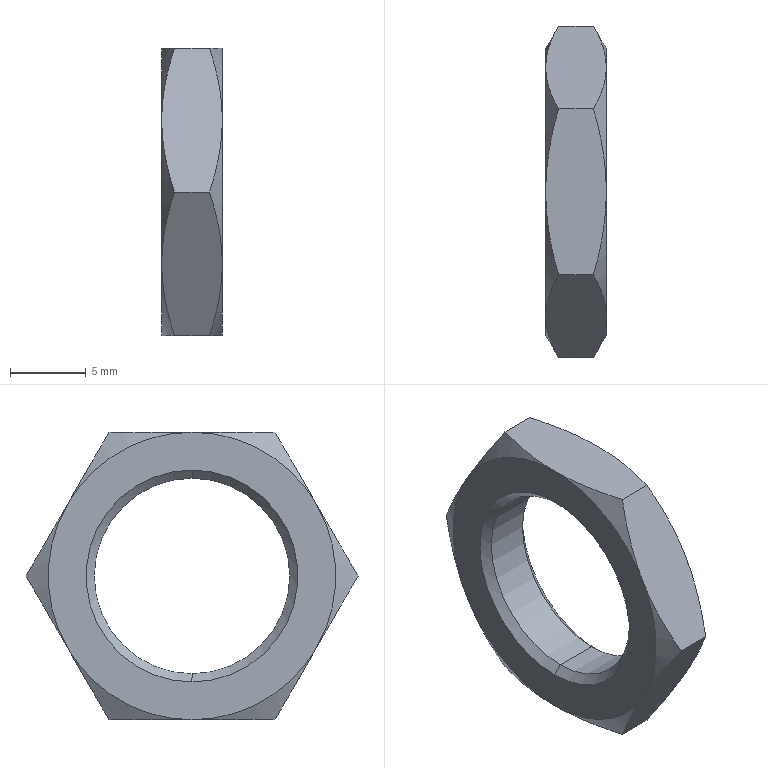Part | SolidWorks | features RefAxis 3, RevCut 2, 3DProfileFeature 1, Extrusion 1 | 1 solid | 26 faces | box 4 x 21.939 x 19 mm | volume 699.231 mm3 | cone 16 | plane 8 | cylinder 2 | commonest cylinder face diameters 12.917 x2
STEP:
#1=CARTESIAN_POINT('',(3.459,0.,6.458));
#2=VERTEX_POINT('',#1);
#3=CARTESIAN_POINT('',(3.459,0.,-6.458));
#4=VERTEX_POINT('',#3);
#5=CARTESIAN_POINT('',(3.459,0.,0.));
#6=DIRECTION('',(1.,0.,0.));
#7=DIRECTION('',(0.,0.,-1.));
#8=AXIS2_PLACEMENT_3D('',#5,#6,#7);
#9=CIRCLE('',#8,6.458);
#10=EDGE_CURVE('',#2,#4,#9,.T.);
#11=ORIENTED_EDGE('',*,*,#10,.F.);
#12=CARTESIAN_POINT('',(4.,0.,7.));
#13=VERTEX_POINT('',#12);
#14=CARTESIAN_POINT('',(4.,0.,7.));
#15=DIRECTION('',(0.7071,0.,0.7071));
#16=VECTOR('',#15,1000.);
#17=LINE('',#14,#16);
#18=EDGE_CURVE('',#2,#13,#17,.T.);
#19=ORIENTED_EDGE('',*,*,#18,.T.);
#20=CARTESIAN_POINT('',(4.,0.,-7.));
#21=VERTEX_POINT('',#20);
#22=CARTESIAN_POINT('',(4.,0.,0.));
#23=DIRECTION('',(1.,0.,0.));
#24=DIRECTION('',(0.,0.,-1.));
#25=AXIS2_PLACEMENT_3D('',#22,#23,#24);
#26=CIRCLE('',#25,7.);
#27=EDGE_CURVE('',#13,#21,#26,.T.);
#28=ORIENTED_EDGE('',*,*,#27,.T.);
#29=CARTESIAN_POINT('',(4.,0.,-7.));
#30=DIRECTION('',(0.7071,0.,-0.7071));
#31=VECTOR('',#30,1000.);
#32=LINE('',#29,#31);
#33=EDGE_CURVE('',#4,#21,#32,.T.);
#34=ORIENTED_EDGE('',*,*,#33,.F.);
#35=EDGE_LOOP('',(#11,#19,#28,#34));
#36=FACE_OUTER_BOUND('',#35,.T.);
#37=CARTESIAN_POINT('',(4.,0.,0.));
#38=DIRECTION('',(1.,0.,0.));
#39=DIRECTION('',(0.,0.,-1.));
#40=AXIS2_PLACEMENT_3D('',#37,#38,#39);
#41=CONICAL_SURFACE('',#40,7.,0.7854);
#42=ADVANCED_FACE('',(#36),#41,.F.);
#43=CARTESIAN_POINT('',(0.5415,0.,6.458));
#44=VERTEX_POINT('',#43);
#45=CARTESIAN_POINT('',(0.5415,0.,-6.458));
#46=VERTEX_POINT('',#45);
#47=CARTESIAN_POINT('',(0.5415,0.,0.));
#48=DIRECTION('',(1.,0.,0.));
#49=DIRECTION('',(0.,0.,-1.));
#50=AXIS2_PLACEMENT_3D('',#47,#48,#49);
#51=CIRCLE('',#50,6.458);
#52=EDGE_CURVE('',#44,#46,#51,.T.);
#53=ORIENTED_EDGE('',*,*,#52,.F.);
#54=CARTESIAN_POINT('',(4.,0.,6.458));
#55=DIRECTION('',(1.,0.,0.));
#56=VECTOR('',#55,1000.);
#57=LINE('',#54,#56);
#58=EDGE_CURVE('',#44,#2,#57,.T.);
#59=ORIENTED_EDGE('',*,*,#58,.T.);
#60=ORIENTED_EDGE('',*,*,#10,.T.);
#61=CARTESIAN_POINT('',(4.,0.,-6.458));
#62=DIRECTION('',(1.,0.,0.));
#63=VECTOR('',#62,1000.);
#64=LINE('',#61,#63);
#65=EDGE_CURVE('',#46,#4,#64,.T.);
#66=ORIENTED_EDGE('',*,*,#65,.F.);
#67=EDGE_LOOP('',(#53,#59,#60,#66));
#68=FACE_OUTER_BOUND('',#67,.T.);
#69=CARTESIAN_POINT('',(4.,0.,0.));
#70=DIRECTION('',(1.,0.,0.));
#71=DIRECTION('',(0.,0.,-1.));
#72=AXIS2_PLACEMENT_3D('',#69,#70,#71);
#73=CYLINDRICAL_SURFACE('',#72,6.458);
#74=ADVANCED_FACE('',(#68),#73,.F.);
#75=ORIENTED_EDGE('',*,*,#52,.T.);
#76=CARTESIAN_POINT('',(0.,0.,-7.));
#77=VERTEX_POINT('',#76);
#78=CARTESIAN_POINT('',(0.5415,0.,-6.458));
#79=DIRECTION('',(-0.7071,0.,-0.7071));
#80=VECTOR('',#79,1000.);
#81=LINE('',#78,#80);
#82=EDGE_CURVE('',#46,#77,#81,.T.);
#83=ORIENTED_EDGE('',*,*,#82,.T.);
#84=CARTESIAN_POINT('',(0.,0.,7.));
#85=VERTEX_POINT('',#84);
#86=CARTESIAN_POINT('',(0.,0.,0.));
#87=DIRECTION('',(1.,0.,0.));
#88=DIRECTION('',(0.,0.,-1.));
#89=AXIS2_PLACEMENT_3D('',#86,#87,#88);
#90=CIRCLE('',#89,7.);
#91=EDGE_CURVE('',#85,#77,#90,.T.);
#92=ORIENTED_EDGE('',*,*,#91,.F.);
#93=CARTESIAN_POINT('',(0.5415,0.,6.458));
#94=DIRECTION('',(-0.7071,0.,0.7071));
#95=VECTOR('',#94,1000.);
#96=LINE('',#93,#95);
#97=EDGE_CURVE('',#44,#85,#96,.T.);
#98=ORIENTED_EDGE('',*,*,#97,.F.);
#99=EDGE_LOOP('',(#75,#83,#92,#98));
#100=FACE_OUTER_BOUND('',#99,.T.);
#101=CARTESIAN_POINT('',(0.5415,0.,0.));
#102=DIRECTION('',(-1.,0.,0.));
#103=DIRECTION('',(0.,0.,1.));
#104=AXIS2_PLACEMENT_3D('',#101,#102,#103);
#105=CONICAL_SURFACE('',#104,6.458,0.7854);
#106=ADVANCED_FACE('',(#100),#105,.F.);
#107=CARTESIAN_POINT('',(4.,0.,0.));
#108=DIRECTION('',(1.,0.,0.));
#109=DIRECTION('',(0.,0.,-1.));
#110=AXIS2_PLACEMENT_3D('',#107,#108,#109);
#111=CIRCLE('',#110,7.);
#112=EDGE_CURVE('',#21,#13,#111,.T.);
#113=ORIENTED_EDGE('',*,*,#112,.F.);
#114=ORIENTED_EDGE('',*,*,#27,.F.);
#115=EDGE_LOOP('',(#113,#114));
#116=FACE_BOUND('',#115,.T.);
#117=CARTESIAN_POINT('',(4.,0.,-9.5));
#118=VERTEX_POINT('',#117);
#119=CARTESIAN_POINT('',(4.,-8.227,-4.75));
#120=VERTEX_POINT('',#119);
#121=CARTESIAN_POINT('',(4.,0.,0.));
#122=DIRECTION('',(-1.,0.,0.));
#123=DIRECTION('',(0.,0.,-1.));
#124=AXIS2_PLACEMENT_3D('',#121,#122,#123);
#125=CIRCLE('',#124,9.5);
#126=EDGE_CURVE('',#118,#120,#125,.T.);
#127=ORIENTED_EDGE('',*,*,#126,.F.);
#128=CARTESIAN_POINT('',(4.,8.227,-4.75));
#129=VERTEX_POINT('',#128);
#130=CARTESIAN_POINT('',(4.,0.,0.));
#131=DIRECTION('',(1.,0.,0.));
#132=DIRECTION('',(0.,0.,-1.));
#133=AXIS2_PLACEMENT_3D('',#130,#131,#132);
#134=CIRCLE('',#133,9.5);
#135=EDGE_CURVE('',#118,#129,#134,.T.);
#136=ORIENTED_EDGE('',*,*,#135,.T.);
#137=CARTESIAN_POINT('',(4.,8.227,4.75));
#138=VERTEX_POINT('',#137);
#139=CARTESIAN_POINT('',(4.,0.,0.));
#140=DIRECTION('',(-1.,0.,0.));
#141=DIRECTION('',(0.,0.,-1.));
#142=AXIS2_PLACEMENT_3D('',#139,#140,#141);
#143=CIRCLE('',#142,9.5);
#144=EDGE_CURVE('',#138,#129,#143,.T.);
#145=ORIENTED_EDGE('',*,*,#144,.F.);
#146=CARTESIAN_POINT('',(4.,0.,9.5));
#147=VERTEX_POINT('',#146);
#148=CARTESIAN_POINT('',(4.,0.,0.));
#149=DIRECTION('',(-1.,0.,0.));
#150=DIRECTION('',(0.,0.,-1.));
#151=AXIS2_PLACEMENT_3D('',#148,#149,#150);
#152=CIRCLE('',#151,9.5);
#153=EDGE_CURVE('',#147,#138,#152,.T.);
#154=ORIENTED_EDGE('',*,*,#153,.F.);
#155=CARTESIAN_POINT('',(4.,-8.227,4.75));
#156=VERTEX_POINT('',#155);
#157=CARTESIAN_POINT('',(4.,0.,0.));
#158=DIRECTION('',(-1.,0.,0.));
#159=DIRECTION('',(0.,0.,-1.));
#160=AXIS2_PLACEMENT_3D('',#157,#158,#159);
#161=CIRCLE('',#160,9.5);
#162=EDGE_CURVE('',#156,#147,#161,.T.);
#163=ORIENTED_EDGE('',*,*,#162,.F.);
#164=CARTESIAN_POINT('',(4.,0.,0.));
#165=DIRECTION('',(-1.,0.,0.));
#166=DIRECTION('',(0.,0.,-1.));
#167=AXIS2_PLACEMENT_3D('',#164,#165,#166);
#168=CIRCLE('',#167,9.5);
#169=EDGE_CURVE('',#120,#156,#168,.T.);
#170=ORIENTED_EDGE('',*,*,#169,.F.);
#171=EDGE_LOOP('',(#127,#136,#145,#154,#163,#170));
#172=FACE_OUTER_BOUND('',#171,.T.);
#173=CARTESIAN_POINT('',(4.,5.485,9.5));
#174=DIRECTION('',(1.,0.,0.));
#175=DIRECTION('',(0.,0.,-1.));
#176=AXIS2_PLACEMENT_3D('',#173,#174,#175);
#177=PLANE('',#176);
#178=ADVANCED_FACE('',(#116,#172),#177,.T.);
#179=CARTESIAN_POINT('',(3.151,5.485,-9.5));
#180=VERTEX_POINT('',#179);
#181=CARTESIAN_POINT('',(4.,8.227,-4.75));
#182=CARTESIAN_POINT('',(4.,7.995,-5.153));
#183=CARTESIAN_POINT('',(3.98,7.761,-5.558));
#184=CARTESIAN_POINT('',(3.902,7.298,-6.359));
#185=CARTESIAN_POINT('',(3.845,7.069,-6.757));
#186=CARTESIAN_POINT('',(3.623,6.384,-7.943));
#187=CARTESIAN_POINT('',(3.41,5.932,-8.725));
#188=CARTESIAN_POINT('',(3.151,5.485,-9.5));
#189=B_SPLINE_CURVE_WITH_KNOTS('',3,(#181,#182,#183,#184,#185,#186,#187,#188),.UNSPECIFIED.,.F.,.F.,(4,2,2,4),(0.00555,0.006932,0.008314,0.01108),.UNSPECIFIED.);
#190=EDGE_CURVE('',#129,#180,#189,.T.);
#191=ORIENTED_EDGE('',*,*,#190,.F.);
#192=ORIENTED_EDGE('',*,*,#135,.F.);
#193=CARTESIAN_POINT('',(3.151,5.485,-9.5));
#194=CARTESIAN_POINT('',(3.408,4.598,-9.5));
#195=CARTESIAN_POINT('',(3.621,3.699,-9.5));
#196=CARTESIAN_POINT('',(3.918,1.868,-9.5));
#197=CARTESIAN_POINT('',(4.,0.928,-9.5));
#198=CARTESIAN_POINT('',(4.,0.,-9.5));
#199=B_SPLINE_CURVE_WITH_KNOTS('',3,(#193,#194,#195,#196,#197,#198),.UNSPECIFIED.,.F.,.F.,(4,2,4),(0.02456,0.02734,0.03012),.UNSPECIFIED.);
#200=EDGE_CURVE('',#180,#118,#199,.T.);
#201=ORIENTED_EDGE('',*,*,#200,.F.);
#202=EDGE_LOOP('',(#191,#192,#201));
#203=FACE_OUTER_BOUND('',#202,.T.);
#204=CARTESIAN_POINT('',(2.,0.,0.));
#205=DIRECTION('',(-1.,0.,0.));
#206=DIRECTION('',(0.,0.,1.));
#207=AXIS2_PLACEMENT_3D('',#204,#205,#206);
#208=CONICAL_SURFACE('',#207,12.964,1.047);
#209=ADVANCED_FACE('',(#203),#208,.T.);
#210=ORIENTED_EDGE('',*,*,#144,.T.);
#211=CARTESIAN_POINT('',(3.151,10.97,0.));
#212=VERTEX_POINT('',#211);
#213=CARTESIAN_POINT('',(3.151,10.97,0.));
#214=CARTESIAN_POINT('',(3.411,10.521,-0.777));
#215=CARTESIAN_POINT('',(3.624,10.069,-1.56));
#216=CARTESIAN_POINT('',(3.919,9.156,-3.142));
#217=CARTESIAN_POINT('',(4.,8.694,-3.941));
#218=CARTESIAN_POINT('',(4.,8.227,-4.75));
#219=B_SPLINE_CURVE_WITH_KNOTS('',3,(#213,#214,#215,#216,#217,#218),.UNSPECIFIED.,.F.,.F.,(4,2,4),(0.000000238,0.002775,0.00555),.UNSPECIFIED.);
#220=EDGE_CURVE('',#212,#129,#219,.T.);
#221=ORIENTED_EDGE('',*,*,#220,.F.);
#222=CARTESIAN_POINT('',(4.,8.227,4.75));
#223=CARTESIAN_POINT('',(4.,8.46,4.347));
#224=CARTESIAN_POINT('',(3.98,8.694,3.942));
#225=CARTESIAN_POINT('',(3.902,9.156,3.141));
#226=CARTESIAN_POINT('',(3.845,9.386,2.743));
#227=CARTESIAN_POINT('',(3.623,10.071,1.557));
#228=CARTESIAN_POINT('',(3.41,10.522,0.7751));
#229=CARTESIAN_POINT('',(3.151,10.97,0.));
#230=B_SPLINE_CURVE_WITH_KNOTS('',3,(#222,#223,#224,#225,#226,#227,#228,#229),.UNSPECIFIED.,.F.,.F.,(4,2,2,4),(0.00555,0.006932,0.008314,0.01108),.UNSPECIFIED.);
#231=EDGE_CURVE('',#138,#212,#230,.T.);
#232=ORIENTED_EDGE('',*,*,#231,.F.);
#233=EDGE_LOOP('',(#210,#221,#232));
#234=FACE_OUTER_BOUND('',#233,.T.);
#235=CARTESIAN_POINT('',(2.,0.,0.));
#236=DIRECTION('',(-1.,0.,0.));
#237=DIRECTION('',(0.,0.,1.));
#238=AXIS2_PLACEMENT_3D('',#235,#236,#237);
#239=CONICAL_SURFACE('',#238,12.964,1.047);
#240=ADVANCED_FACE('',(#234),#239,.T.);
#241=ORIENTED_EDGE('',*,*,#153,.T.);
#242=CARTESIAN_POINT('',(3.151,5.485,9.5));
#243=VERTEX_POINT('',#242);
#244=CARTESIAN_POINT('',(3.151,5.485,9.5));
#245=CARTESIAN_POINT('',(3.411,5.933,8.723));
#246=CARTESIAN_POINT('',(3.624,6.385,7.94));
#247=CARTESIAN_POINT('',(3.919,7.299,6.358));
#248=CARTESIAN_POINT('',(4.,7.76,5.559));
#249=CARTESIAN_POINT('',(4.,8.227,4.75));
#250=B_SPLINE_CURVE_WITH_KNOTS('',3,(#244,#245,#246,#247,#248,#249),.UNSPECIFIED.,.F.,.F.,(4,2,4),(0.000000238,0.002775,0.00555),.UNSPECIFIED.);
#251=EDGE_CURVE('',#243,#138,#250,.T.);
#252=ORIENTED_EDGE('',*,*,#251,.F.);
#253=CARTESIAN_POINT('',(4.,0.,9.5));
#254=CARTESIAN_POINT('',(4.,0.928,9.5));
#255=CARTESIAN_POINT('',(3.918,1.868,9.5));
#256=CARTESIAN_POINT('',(3.621,3.699,9.5));
#257=CARTESIAN_POINT('',(3.408,4.598,9.5));
#258=CARTESIAN_POINT('',(3.151,5.485,9.5));
#259=B_SPLINE_CURVE_WITH_KNOTS('',3,(#253,#254,#255,#256,#257,#258),.UNSPECIFIED.,.F.,.F.,(4,2,4),(0.01551,0.01829,0.02107),.UNSPECIFIED.);
#260=EDGE_CURVE('',#147,#243,#259,.T.);
#261=ORIENTED_EDGE('',*,*,#260,.F.);
#262=EDGE_LOOP('',(#241,#252,#261));
#263=FACE_OUTER_BOUND('',#262,.T.);
#264=CARTESIAN_POINT('',(2.,0.,0.));
#265=DIRECTION('',(-1.,0.,0.));
#266=DIRECTION('',(0.,0.,1.));
#267=AXIS2_PLACEMENT_3D('',#264,#265,#266);
#268=CONICAL_SURFACE('',#267,12.964,1.047);
#269=ADVANCED_FACE('',(#263),#268,.T.);
#270=ORIENTED_EDGE('',*,*,#162,.T.);
#271=CARTESIAN_POINT('',(3.151,-5.485,9.5));
#272=VERTEX_POINT('',#271);
#273=CARTESIAN_POINT('',(3.151,-5.485,9.5));
#274=CARTESIAN_POINT('',(3.409,-4.592,9.5));
#275=CARTESIAN_POINT('',(3.625,-3.679,9.5));
#276=CARTESIAN_POINT('',(3.92,-1.848,9.5));
#277=CARTESIAN_POINT('',(4.,-0.9274,9.5));
#278=CARTESIAN_POINT('',(4.,0.,9.5));
#279=B_SPLINE_CURVE_WITH_KNOTS('',3,(#273,#274,#275,#276,#277,#278),.UNSPECIFIED.,.F.,.F.,(4,2,4),(0.009964,0.01274,0.01551),.UNSPECIFIED.);
#280=EDGE_CURVE('',#272,#147,#279,.T.);
#281=ORIENTED_EDGE('',*,*,#280,.F.);
#282=CARTESIAN_POINT('',(4.,-8.227,4.75));
#283=CARTESIAN_POINT('',(4.,-7.995,5.153));
#284=CARTESIAN_POINT('',(3.98,-7.761,5.558));
#285=CARTESIAN_POINT('',(3.902,-7.298,6.359));
#286=CARTESIAN_POINT('',(3.845,-7.069,6.757));
#287=CARTESIAN_POINT('',(3.623,-6.384,7.943));
#288=CARTESIAN_POINT('',(3.41,-5.932,8.725));
#289=CARTESIAN_POINT('',(3.151,-5.485,9.5));
#290=B_SPLINE_CURVE_WITH_KNOTS('',3,(#282,#283,#284,#285,#286,#287,#288,#289),.UNSPECIFIED.,.F.,.F.,(4,2,2,4),(0.00555,0.006932,0.008314,0.01108),.UNSPECIFIED.);
#291=EDGE_CURVE('',#156,#272,#290,.T.);
#292=ORIENTED_EDGE('',*,*,#291,.F.);
#293=EDGE_LOOP('',(#270,#281,#292));
#294=FACE_OUTER_BOUND('',#293,.T.);
#295=CARTESIAN_POINT('',(2.,0.,0.));
#296=DIRECTION('',(-1.,0.,0.));
#297=DIRECTION('',(0.,0.,1.));
#298=AXIS2_PLACEMENT_3D('',#295,#296,#297);
#299=CONICAL_SURFACE('',#298,12.964,1.047);
#300=ADVANCED_FACE('',(#294),#299,.T.);
#301=CARTESIAN_POINT('',(3.151,-10.97,0.));
#302=VERTEX_POINT('',#301);
#303=CARTESIAN_POINT('',(4.,-8.227,-4.75));
#304=CARTESIAN_POINT('',(4.,-8.46,-4.347));
#305=CARTESIAN_POINT('',(3.98,-8.694,-3.942));
#306=CARTESIAN_POINT('',(3.902,-9.156,-3.141));
#307=CARTESIAN_POINT('',(3.845,-9.386,-2.743));
#308=CARTESIAN_POINT('',(3.623,-10.071,-1.557));
#309=CARTESIAN_POINT('',(3.41,-10.522,-0.7751));
#310=CARTESIAN_POINT('',(3.151,-10.97,0.));
#311=B_SPLINE_CURVE_WITH_KNOTS('',3,(#303,#304,#305,#306,#307,#308,#309,#310),.UNSPECIFIED.,.F.,.F.,(4,2,2,4),(0.00555,0.006932,0.008314,0.01108),.UNSPECIFIED.);
#312=EDGE_CURVE('',#120,#302,#311,.T.);
#313=ORIENTED_EDGE('',*,*,#312,.F.);
#314=ORIENTED_EDGE('',*,*,#169,.T.);
#315=CARTESIAN_POINT('',(3.151,-10.97,0.));
#316=CARTESIAN_POINT('',(3.411,-10.521,0.777));
#317=CARTESIAN_POINT('',(3.624,-10.069,1.56));
#318=CARTESIAN_POINT('',(3.919,-9.156,3.142));
#319=CARTESIAN_POINT('',(4.,-8.694,3.941));
#320=CARTESIAN_POINT('',(4.,-8.227,4.75));
#321=B_SPLINE_CURVE_WITH_KNOTS('',3,(#315,#316,#317,#318,#319,#320),.UNSPECIFIED.,.F.,.F.,(4,2,4),(0.000000238,0.002775,0.00555),.UNSPECIFIED.);
#322=EDGE_CURVE('',#302,#156,#321,.T.);
#323=ORIENTED_EDGE('',*,*,#322,.F.);
#324=EDGE_LOOP('',(#313,#314,#323));
#325=FACE_OUTER_BOUND('',#324,.T.);
#326=CARTESIAN_POINT('',(2.,0.,0.));
#327=DIRECTION('',(-1.,0.,0.));
#328=DIRECTION('',(0.,0.,1.));
#329=AXIS2_PLACEMENT_3D('',#326,#327,#328);
#330=CONICAL_SURFACE('',#329,12.964,1.047);
#331=ADVANCED_FACE('',(#325),#330,.T.);
#332=CARTESIAN_POINT('',(3.151,-5.485,-9.5));
#333=VERTEX_POINT('',#332);
#334=CARTESIAN_POINT('',(4.,0.,-9.5));
#335=CARTESIAN_POINT('',(4.,-0.9274,-9.5));
#336=CARTESIAN_POINT('',(3.92,-1.848,-9.5));
#337=CARTESIAN_POINT('',(3.625,-3.679,-9.5));
#338=CARTESIAN_POINT('',(3.409,-4.592,-9.5));
#339=CARTESIAN_POINT('',(3.151,-5.485,-9.5));
#340=B_SPLINE_CURVE_WITH_KNOTS('',3,(#334,#335,#336,#337,#338,#339),.UNSPECIFIED.,.F.,.F.,(4,2,4),(0.03012,0.03289,0.03567),.UNSPECIFIED.);
#341=EDGE_CURVE('',#118,#333,#340,.T.);
#342=ORIENTED_EDGE('',*,*,#341,.F.);
#343=ORIENTED_EDGE('',*,*,#126,.T.);
#344=CARTESIAN_POINT('',(3.151,-5.485,-9.5));
#345=CARTESIAN_POINT('',(3.411,-5.933,-8.723));
#346=CARTESIAN_POINT('',(3.624,-6.385,-7.94));
#347=CARTESIAN_POINT('',(3.919,-7.299,-6.358));
#348=CARTESIAN_POINT('',(4.,-7.76,-5.559));
#349=CARTESIAN_POINT('',(4.,-8.227,-4.75));
#350=B_SPLINE_CURVE_WITH_KNOTS('',3,(#344,#345,#346,#347,#348,#349),.UNSPECIFIED.,.F.,.F.,(4,2,4),(0.000000238,0.002775,0.00555),.UNSPECIFIED.);
#351=EDGE_CURVE('',#333,#120,#350,.T.);
#352=ORIENTED_EDGE('',*,*,#351,.F.);
#353=EDGE_LOOP('',(#342,#343,#352));
#354=FACE_OUTER_BOUND('',#353,.T.);
#355=CARTESIAN_POINT('',(2.,0.,0.));
#356=DIRECTION('',(-1.,0.,0.));
#357=DIRECTION('',(0.,0.,1.));
#358=AXIS2_PLACEMENT_3D('',#355,#356,#357);
#359=CONICAL_SURFACE('',#358,12.964,1.047);
#360=ADVANCED_FACE('',(#354),#359,.T.);
#361=CARTESIAN_POINT('',(0.8485,10.97,0.));
#362=VERTEX_POINT('',#361);
#363=CARTESIAN_POINT('',(4.,10.97,0.));
#364=DIRECTION('',(-1.,0.,0.));
#365=VECTOR('',#364,1000.);
#366=LINE('',#363,#365);
#367=EDGE_CURVE('',#212,#362,#366,.T.);
#368=ORIENTED_EDGE('',*,*,#367,.T.);
#369=CARTESIAN_POINT('',(0.,8.227,4.75));
#370=VERTEX_POINT('',#369);
#371=CARTESIAN_POINT('',(0.8485,10.97,0.));
#372=CARTESIAN_POINT('',(0.5895,10.521,0.777));
#373=CARTESIAN_POINT('',(0.3761,10.069,1.56));
#374=CARTESIAN_POINT('',(0.08087,9.156,3.142));
#375=CARTESIAN_POINT('',(0.,8.694,3.941));
#376=CARTESIAN_POINT('',(0.,8.227,4.75));
#377=B_SPLINE_CURVE_WITH_KNOTS('',3,(#371,#372,#373,#374,#375,#376),.UNSPECIFIED.,.F.,.F.,(4,2,4),(0.000000238,0.002775,0.00555),.UNSPECIFIED.);
#378=EDGE_CURVE('',#362,#370,#377,.T.);
#379=ORIENTED_EDGE('',*,*,#378,.T.);
#380=CARTESIAN_POINT('',(0.8485,5.485,9.5));
#381=VERTEX_POINT('',#380);
#382=CARTESIAN_POINT('',(0.,8.227,4.75));
#383=CARTESIAN_POINT('',(0.,7.995,5.153));
#384=CARTESIAN_POINT('',(0.02006,7.761,5.558));
#385=CARTESIAN_POINT('',(0.09767,7.298,6.359));
#386=CARTESIAN_POINT('',(0.1552,7.069,6.757));
#387=CARTESIAN_POINT('',(0.3769,6.384,7.943));
#388=CARTESIAN_POINT('',(0.5901,5.932,8.725));
#389=CARTESIAN_POINT('',(0.8485,5.485,9.5));
#390=B_SPLINE_CURVE_WITH_KNOTS('',3,(#382,#383,#384,#385,#386,#387,#388,#389),.UNSPECIFIED.,.F.,.F.,(4,2,2,4),(0.00555,0.006932,0.008314,0.01108),.UNSPECIFIED.);
#391=EDGE_CURVE('',#370,#381,#390,.T.);
#392=ORIENTED_EDGE('',*,*,#391,.T.);
#393=CARTESIAN_POINT('',(4.,5.485,9.5));
#394=DIRECTION('',(-1.,0.,0.));
#395=VECTOR('',#394,1000.);
#396=LINE('',#393,#395);
#397=EDGE_CURVE('',#243,#381,#396,.T.);
#398=ORIENTED_EDGE('',*,*,#397,.F.);
#399=ORIENTED_EDGE('',*,*,#251,.T.);
#400=ORIENTED_EDGE('',*,*,#231,.T.);
#401=EDGE_LOOP('',(#368,#379,#392,#398,#399,#400));
#402=FACE_OUTER_BOUND('',#401,.T.);
#403=CARTESIAN_POINT('',(4.,10.97,0.));
#404=DIRECTION('',(0.,-0.866,-0.5));
#405=DIRECTION('',(0.,0.5,-0.866));
#406=AXIS2_PLACEMENT_3D('',#403,#404,#405);
#407=PLANE('',#406);
#408=ADVANCED_FACE('',(#402),#407,.F.);
#409=ORIENTED_EDGE('',*,*,#397,.T.);
#410=CARTESIAN_POINT('',(0.,0.,9.5));
#411=VERTEX_POINT('',#410);
#412=CARTESIAN_POINT('',(0.8485,5.485,9.5));
#413=CARTESIAN_POINT('',(0.5925,4.598,9.5));
#414=CARTESIAN_POINT('',(0.3793,3.699,9.5));
#415=CARTESIAN_POINT('',(0.08199,1.868,9.5));
#416=CARTESIAN_POINT('',(0.,0.928,9.5));
#417=CARTESIAN_POINT('',(0.,0.,9.5));
#418=B_SPLINE_CURVE_WITH_KNOTS('',3,(#412,#413,#414,#415,#416,#417),.UNSPECIFIED.,.F.,.F.,(4,2,4),(0.02456,0.02734,0.03012),.UNSPECIFIED.);
#419=EDGE_CURVE('',#381,#411,#418,.T.);
#420=ORIENTED_EDGE('',*,*,#419,.T.);
#421=CARTESIAN_POINT('',(0.8485,-5.485,9.5));
#422=VERTEX_POINT('',#421);
#423=CARTESIAN_POINT('',(0.,0.,9.5));
#424=CARTESIAN_POINT('',(0.,-0.9274,9.5));
#425=CARTESIAN_POINT('',(0.07975,-1.848,9.5));
#426=CARTESIAN_POINT('',(0.375,-3.679,9.5));
#427=CARTESIAN_POINT('',(0.5908,-4.592,9.5));
#428=CARTESIAN_POINT('',(0.8485,-5.485,9.5));
#429=B_SPLINE_CURVE_WITH_KNOTS('',3,(#423,#424,#425,#426,#427,#428),.UNSPECIFIED.,.F.,.F.,(4,2,4),(0.03012,0.03289,0.03567),.UNSPECIFIED.);
#430=EDGE_CURVE('',#411,#422,#429,.T.);
#431=ORIENTED_EDGE('',*,*,#430,.T.);
#432=CARTESIAN_POINT('',(4.,-5.485,9.5));
#433=DIRECTION('',(-1.,0.,0.));
#434=VECTOR('',#433,1000.);
#435=LINE('',#432,#434);
#436=EDGE_CURVE('',#272,#422,#435,.T.);
#437=ORIENTED_EDGE('',*,*,#436,.F.);
#438=ORIENTED_EDGE('',*,*,#280,.T.);
#439=ORIENTED_EDGE('',*,*,#260,.T.);
#440=EDGE_LOOP('',(#409,#420,#431,#437,#438,#439));
#441=FACE_OUTER_BOUND('',#440,.T.);
#442=CARTESIAN_POINT('',(4.,5.485,9.5));
#443=DIRECTION('',(0.,0.,-1.));
#444=DIRECTION('',(-1.,0.,0.));
#445=AXIS2_PLACEMENT_3D('',#442,#443,#444);
#446=PLANE('',#445);
#447=ADVANCED_FACE('',(#441),#446,.F.);
#448=ORIENTED_EDGE('',*,*,#436,.T.);
#449=CARTESIAN_POINT('',(0.,-8.227,4.75));
#450=VERTEX_POINT('',#449);
#451=CARTESIAN_POINT('',(0.8485,-5.485,9.5));
#452=CARTESIAN_POINT('',(0.5895,-5.933,8.723));
#453=CARTESIAN_POINT('',(0.3761,-6.385,7.94));
#454=CARTESIAN_POINT('',(0.08087,-7.299,6.358));
#455=CARTESIAN_POINT('',(0.,-7.76,5.559));
#456=CARTESIAN_POINT('',(0.,-8.227,4.75));
#457=B_SPLINE_CURVE_WITH_KNOTS('',3,(#451,#452,#453,#454,#455,#456),.UNSPECIFIED.,.F.,.F.,(4,2,4),(0.000000238,0.002775,0.00555),.UNSPECIFIED.);
#458=EDGE_CURVE('',#422,#450,#457,.T.);
#459=ORIENTED_EDGE('',*,*,#458,.T.);
#460=CARTESIAN_POINT('',(0.8485,-10.97,0.));
#461=VERTEX_POINT('',#460);
#462=CARTESIAN_POINT('',(0.,-8.227,4.75));
#463=CARTESIAN_POINT('',(0.,-8.46,4.347));
#464=CARTESIAN_POINT('',(0.02006,-8.694,3.942));
#465=CARTESIAN_POINT('',(0.09767,-9.156,3.141));
#466=CARTESIAN_POINT('',(0.1552,-9.386,2.743));
#467=CARTESIAN_POINT('',(0.3769,-10.071,1.557));
#468=CARTESIAN_POINT('',(0.5901,-10.522,0.7751));
#469=CARTESIAN_POINT('',(0.8485,-10.97,0.));
#470=B_SPLINE_CURVE_WITH_KNOTS('',3,(#462,#463,#464,#465,#466,#467,#468,#469),.UNSPECIFIED.,.F.,.F.,(4,2,2,4),(0.00555,0.006932,0.008314,0.01108),.UNSPECIFIED.);
#471=EDGE_CURVE('',#450,#461,#470,.T.);
#472=ORIENTED_EDGE('',*,*,#471,.T.);
#473=CARTESIAN_POINT('',(4.,-10.97,0.));
#474=DIRECTION('',(-1.,0.,0.));
#475=VECTOR('',#474,1000.);
#476=LINE('',#473,#475);
#477=EDGE_CURVE('',#302,#461,#476,.T.);
#478=ORIENTED_EDGE('',*,*,#477,.F.);
#479=ORIENTED_EDGE('',*,*,#322,.T.);
#480=ORIENTED_EDGE('',*,*,#291,.T.);
#481=EDGE_LOOP('',(#448,#459,#472,#478,#479,#480));
#482=FACE_OUTER_BOUND('',#481,.T.);
#483=CARTESIAN_POINT('',(4.,-5.485,9.5));
#484=DIRECTION('',(0.,0.866,-0.5));
#485=DIRECTION('',(0.,0.5,0.866));
#486=AXIS2_PLACEMENT_3D('',#483,#484,#485);
#487=PLANE('',#486);
#488=ADVANCED_FACE('',(#482),#487,.F.);
#489=ORIENTED_EDGE('',*,*,#477,.T.);
#490=CARTESIAN_POINT('',(0.,-8.227,-4.75));
#491=VERTEX_POINT('',#490);
#492=CARTESIAN_POINT('',(0.8485,-10.97,0.));
#493=CARTESIAN_POINT('',(0.5895,-10.521,-0.777));
#494=CARTESIAN_POINT('',(0.3761,-10.069,-1.56));
#495=CARTESIAN_POINT('',(0.08087,-9.156,-3.142));
#496=CARTESIAN_POINT('',(0.,-8.694,-3.941));
#497=CARTESIAN_POINT('',(0.,-8.227,-4.75));
#498=B_SPLINE_CURVE_WITH_KNOTS('',3,(#492,#493,#494,#495,#496,#497),.UNSPECIFIED.,.F.,.F.,(4,2,4),(0.000000238,0.002775,0.00555),.UNSPECIFIED.);
#499=EDGE_CURVE('',#461,#491,#498,.T.);
#500=ORIENTED_EDGE('',*,*,#499,.T.);
#501=CARTESIAN_POINT('',(0.8485,-5.485,-9.5));
#502=VERTEX_POINT('',#501);
#503=CARTESIAN_POINT('',(0.,-8.227,-4.75));
#504=CARTESIAN_POINT('',(0.,-7.995,-5.153));
#505=CARTESIAN_POINT('',(0.02006,-7.761,-5.558));
#506=CARTESIAN_POINT('',(0.09767,-7.298,-6.359));
#507=CARTESIAN_POINT('',(0.1552,-7.069,-6.757));
#508=CARTESIAN_POINT('',(0.3769,-6.384,-7.943));
#509=CARTESIAN_POINT('',(0.5901,-5.932,-8.725));
#510=CARTESIAN_POINT('',(0.8485,-5.485,-9.5));
#511=B_SPLINE_CURVE_WITH_KNOTS('',3,(#503,#504,#505,#506,#507,#508,#509,#510),.UNSPECIFIED.,.F.,.F.,(4,2,2,4),(0.00555,0.006932,0.008314,0.01108),.UNSPECIFIED.);
#512=EDGE_CURVE('',#491,#502,#511,.T.);
#513=ORIENTED_EDGE('',*,*,#512,.T.);
#514=CARTESIAN_POINT('',(4.,-5.485,-9.5));
#515=DIRECTION('',(-1.,0.,0.));
#516=VECTOR('',#515,1000.);
#517=LINE('',#514,#516);
#518=EDGE_CURVE('',#333,#502,#517,.T.);
#519=ORIENTED_EDGE('',*,*,#518,.F.);
#520=ORIENTED_EDGE('',*,*,#351,.T.);
#521=ORIENTED_EDGE('',*,*,#312,.T.);
#522=EDGE_LOOP('',(#489,#500,#513,#519,#520,#521));
#523=FACE_OUTER_BOUND('',#522,.T.);
#524=CARTESIAN_POINT('',(4.,-10.97,0.));
#525=DIRECTION('',(0.,0.866,0.5));
#526=DIRECTION('',(0.,-0.5,0.866));
#527=AXIS2_PLACEMENT_3D('',#524,#525,#526);
#528=PLANE('',#527);
#529=ADVANCED_FACE('',(#523),#528,.F.);
#530=ORIENTED_EDGE('',*,*,#518,.T.);
#531=CARTESIAN_POINT('',(0.,0.,-9.5));
#532=VERTEX_POINT('',#531);
#533=CARTESIAN_POINT('',(0.8485,-5.485,-9.5));
#534=CARTESIAN_POINT('',(0.5908,-4.592,-9.5));
#535=CARTESIAN_POINT('',(0.375,-3.679,-9.5));
#536=CARTESIAN_POINT('',(0.07975,-1.848,-9.5));
#537=CARTESIAN_POINT('',(0.,-0.9274,-9.5));
#538=CARTESIAN_POINT('',(0.,0.,-9.5));
#539=B_SPLINE_CURVE_WITH_KNOTS('',3,(#533,#534,#535,#536,#537,#538),.UNSPECIFIED.,.F.,.F.,(4,2,4),(0.009964,0.01274,0.01551),.UNSPECIFIED.);
#540=EDGE_CURVE('',#502,#532,#539,.T.);
#541=ORIENTED_EDGE('',*,*,#540,.T.);
#542=CARTESIAN_POINT('',(0.8485,5.485,-9.5));
#543=VERTEX_POINT('',#542);
#544=CARTESIAN_POINT('',(0.,0.,-9.5));
#545=CARTESIAN_POINT('',(0.,0.928,-9.5));
#546=CARTESIAN_POINT('',(0.08199,1.868,-9.5));
#547=CARTESIAN_POINT('',(0.3793,3.699,-9.5));
#548=CARTESIAN_POINT('',(0.5925,4.598,-9.5));
#549=CARTESIAN_POINT('',(0.8485,5.485,-9.5));
#550=B_SPLINE_CURVE_WITH_KNOTS('',3,(#544,#545,#546,#547,#548,#549),.UNSPECIFIED.,.F.,.F.,(4,2,4),(0.01551,0.01829,0.02107),.UNSPECIFIED.);
#551=EDGE_CURVE('',#532,#543,#550,.T.);
#552=ORIENTED_EDGE('',*,*,#551,.T.);
#553=CARTESIAN_POINT('',(4.,5.485,-9.5));
#554=DIRECTION('',(-1.,0.,0.));
#555=VECTOR('',#554,1000.);
#556=LINE('',#553,#555);
#557=EDGE_CURVE('',#180,#543,#556,.T.);
#558=ORIENTED_EDGE('',*,*,#557,.F.);
#559=ORIENTED_EDGE('',*,*,#200,.T.);
#560=ORIENTED_EDGE('',*,*,#341,.T.);
#561=EDGE_LOOP('',(#530,#541,#552,#558,#559,#560));
#562=FACE_OUTER_BOUND('',#561,.T.);
#563=CARTESIAN_POINT('',(4.,-5.485,-9.5));
#564=DIRECTION('',(0.,0.,1.));
#565=DIRECTION('',(1.,0.,0.));
#566=AXIS2_PLACEMENT_3D('',#563,#564,#565);
#567=PLANE('',#566);
#568=ADVANCED_FACE('',(#562),#567,.F.);
#569=ORIENTED_EDGE('',*,*,#557,.T.);
#570=CARTESIAN_POINT('',(0.,8.227,-4.75));
#571=VERTEX_POINT('',#570);
#572=CARTESIAN_POINT('',(0.8485,5.485,-9.5));
#573=CARTESIAN_POINT('',(0.5895,5.933,-8.723));
#574=CARTESIAN_POINT('',(0.3761,6.385,-7.94));
#575=CARTESIAN_POINT('',(0.08087,7.299,-6.358));
#576=CARTESIAN_POINT('',(0.,7.76,-5.559));
#577=CARTESIAN_POINT('',(0.,8.227,-4.75));
#578=B_SPLINE_CURVE_WITH_KNOTS('',3,(#572,#573,#574,#575,#576,#577),.UNSPECIFIED.,.F.,.F.,(4,2,4),(0.000000238,0.002775,0.00555),.UNSPECIFIED.);
#579=EDGE_CURVE('',#543,#571,#578,.T.);
#580=ORIENTED_EDGE('',*,*,#579,.T.);
#581=CARTESIAN_POINT('',(0.,8.227,-4.75));
#582=CARTESIAN_POINT('',(0.,8.46,-4.347));
#583=CARTESIAN_POINT('',(0.02006,8.694,-3.942));
#584=CARTESIAN_POINT('',(0.09767,9.156,-3.141));
#585=CARTESIAN_POINT('',(0.1552,9.386,-2.743));
#586=CARTESIAN_POINT('',(0.3769,10.071,-1.557));
#587=CARTESIAN_POINT('',(0.5901,10.522,-0.7751));
#588=CARTESIAN_POINT('',(0.8485,10.97,0.));
#589=B_SPLINE_CURVE_WITH_KNOTS('',3,(#581,#582,#583,#584,#585,#586,#587,#588),.UNSPECIFIED.,.F.,.F.,(4,2,2,4),(0.00555,0.006932,0.008314,0.01108),.UNSPECIFIED.);
#590=EDGE_CURVE('',#571,#362,#589,.T.);
#591=ORIENTED_EDGE('',*,*,#590,.T.);
#592=ORIENTED_EDGE('',*,*,#367,.F.);
#593=ORIENTED_EDGE('',*,*,#220,.T.);
#594=ORIENTED_EDGE('',*,*,#190,.T.);
#595=EDGE_LOOP('',(#569,#580,#591,#592,#593,#594));
#596=FACE_OUTER_BOUND('',#595,.T.);
#597=CARTESIAN_POINT('',(4.,5.485,-9.5));
#598=DIRECTION('',(0.,-0.866,0.5));
#599=DIRECTION('',(0.,-0.5,-0.866));
#600=AXIS2_PLACEMENT_3D('',#597,#598,#599);
#601=PLANE('',#600);
#602=ADVANCED_FACE('',(#596),#601,.F.);
#603=CARTESIAN_POINT('',(0.,0.,0.));
#604=DIRECTION('',(1.,0.,0.));
#605=DIRECTION('',(0.,0.,-1.));
#606=AXIS2_PLACEMENT_3D('',#603,#604,#605);
#607=CIRCLE('',#606,9.5);
#608=EDGE_CURVE('',#532,#571,#607,.T.);
#609=ORIENTED_EDGE('',*,*,#608,.T.);
#610=ORIENTED_EDGE('',*,*,#579,.F.);
#611=ORIENTED_EDGE('',*,*,#551,.F.);
#612=EDGE_LOOP('',(#609,#610,#611));
#613=FACE_OUTER_BOUND('',#612,.T.);
#614=CARTESIAN_POINT('',(0.,0.,0.));
#615=DIRECTION('',(1.,0.,0.));
#616=DIRECTION('',(0.,0.,-1.));
#617=AXIS2_PLACEMENT_3D('',#614,#615,#616);
#618=CONICAL_SURFACE('',#617,9.5,1.047);
#619=ADVANCED_FACE('',(#613),#618,.T.);
#620=ORIENTED_EDGE('',*,*,#590,.F.);
#621=CARTESIAN_POINT('',(0.,0.,0.));
#622=DIRECTION('',(-1.,0.,0.));
#623=DIRECTION('',(0.,0.,-1.));
#624=AXIS2_PLACEMENT_3D('',#621,#622,#623);
#625=CIRCLE('',#624,9.5);
#626=EDGE_CURVE('',#370,#571,#625,.T.);
#627=ORIENTED_EDGE('',*,*,#626,.F.);
#628=ORIENTED_EDGE('',*,*,#378,.F.);
#629=EDGE_LOOP('',(#620,#627,#628));
#630=FACE_OUTER_BOUND('',#629,.T.);
#631=CARTESIAN_POINT('',(0.,0.,0.));
#632=DIRECTION('',(1.,0.,0.));
#633=DIRECTION('',(0.,0.,-1.));
#634=AXIS2_PLACEMENT_3D('',#631,#632,#633);
#635=CONICAL_SURFACE('',#634,9.5,1.047);
#636=ADVANCED_FACE('',(#630),#635,.T.);
#637=CARTESIAN_POINT('',(0.,0.,0.));
#638=DIRECTION('',(-1.,0.,0.));
#639=DIRECTION('',(0.,0.,-1.));
#640=AXIS2_PLACEMENT_3D('',#637,#638,#639);
#641=CIRCLE('',#640,9.5);
#642=EDGE_CURVE('',#411,#370,#641,.T.);
#643=ORIENTED_EDGE('',*,*,#642,.F.);
#644=ORIENTED_EDGE('',*,*,#419,.F.);
#645=ORIENTED_EDGE('',*,*,#391,.F.);
#646=EDGE_LOOP('',(#643,#644,#645));
#647=FACE_OUTER_BOUND('',#646,.T.);
#648=CARTESIAN_POINT('',(0.,0.,0.));
#649=DIRECTION('',(1.,0.,0.));
#650=DIRECTION('',(0.,0.,-1.));
#651=AXIS2_PLACEMENT_3D('',#648,#649,#650);
#652=CONICAL_SURFACE('',#651,9.5,1.047);
#653=ADVANCED_FACE('',(#647),#652,.T.);
#654=CARTESIAN_POINT('',(0.,0.,0.));
#655=DIRECTION('',(-1.,0.,0.));
#656=DIRECTION('',(0.,0.,-1.));
#657=AXIS2_PLACEMENT_3D('',#654,#655,#656);
#658=CIRCLE('',#657,9.5);
#659=EDGE_CURVE('',#450,#411,#658,.T.);
#660=ORIENTED_EDGE('',*,*,#659,.F.);
#661=ORIENTED_EDGE('',*,*,#458,.F.);
#662=ORIENTED_EDGE('',*,*,#430,.F.);
#663=EDGE_LOOP('',(#660,#661,#662));
#664=FACE_OUTER_BOUND('',#663,.T.);
#665=CARTESIAN_POINT('',(0.,0.,0.));
#666=DIRECTION('',(1.,0.,0.));
#667=DIRECTION('',(0.,0.,-1.));
#668=AXIS2_PLACEMENT_3D('',#665,#666,#667);
#669=CONICAL_SURFACE('',#668,9.5,1.047);
#670=ADVANCED_FACE('',(#664),#669,.T.);
#671=CARTESIAN_POINT('',(0.,0.,0.));
#672=DIRECTION('',(-1.,0.,0.));
#673=DIRECTION('',(0.,0.,-1.));
#674=AXIS2_PLACEMENT_3D('',#671,#672,#673);
#675=CIRCLE('',#674,9.5);
#676=EDGE_CURVE('',#491,#450,#675,.T.);
#677=ORIENTED_EDGE('',*,*,#676,.F.);
#678=ORIENTED_EDGE('',*,*,#499,.F.);
#679=ORIENTED_EDGE('',*,*,#471,.F.);
#680=EDGE_LOOP('',(#677,#678,#679));
#681=FACE_OUTER_BOUND('',#680,.T.);
#682=CARTESIAN_POINT('',(0.,0.,0.));
#683=DIRECTION('',(1.,0.,0.));
#684=DIRECTION('',(0.,0.,-1.));
#685=AXIS2_PLACEMENT_3D('',#682,#683,#684);
#686=CONICAL_SURFACE('',#685,9.5,1.047);
#687=ADVANCED_FACE('',(#681),#686,.T.);
#688=CARTESIAN_POINT('',(0.,0.,0.));
#689=DIRECTION('',(-1.,0.,0.));
#690=DIRECTION('',(0.,0.,-1.));
#691=AXIS2_PLACEMENT_3D('',#688,#689,#690);
#692=CIRCLE('',#691,9.5);
#693=EDGE_CURVE('',#532,#491,#692,.T.);
#694=ORIENTED_EDGE('',*,*,#693,.F.);
#695=ORIENTED_EDGE('',*,*,#540,.F.);
#696=ORIENTED_EDGE('',*,*,#512,.F.);
#697=EDGE_LOOP('',(#694,#695,#696));
#698=FACE_OUTER_BOUND('',#697,.T.);
#699=CARTESIAN_POINT('',(0.,0.,0.));
#700=DIRECTION('',(1.,0.,0.));
#701=DIRECTION('',(0.,0.,-1.));
#702=AXIS2_PLACEMENT_3D('',#699,#700,#701);
#703=CONICAL_SURFACE('',#702,9.5,1.047);
#704=ADVANCED_FACE('',(#698),#703,.T.);
#705=ORIENTED_EDGE('',*,*,#91,.T.);
#706=CARTESIAN_POINT('',(0.,0.,0.));
#707=DIRECTION('',(1.,0.,0.));
#708=DIRECTION('',(0.,0.,-1.));
#709=AXIS2_PLACEMENT_3D('',#706,#707,#708);
#710=CIRCLE('',#709,7.);
#711=EDGE_CURVE('',#77,#85,#710,.T.);
#712=ORIENTED_EDGE('',*,*,#711,.T.);
#713=EDGE_LOOP('',(#705,#712));
#714=FACE_BOUND('',#713,.T.);
#715=ORIENTED_EDGE('',*,*,#608,.F.);
#716=ORIENTED_EDGE('',*,*,#693,.T.);
#717=ORIENTED_EDGE('',*,*,#676,.T.);
#718=ORIENTED_EDGE('',*,*,#659,.T.);
#719=ORIENTED_EDGE('',*,*,#642,.T.);
#720=ORIENTED_EDGE('',*,*,#626,.T.);
#721=EDGE_LOOP('',(#715,#716,#717,#718,#719,#720));
#722=FACE_OUTER_BOUND('',#721,.T.);
#723=CARTESIAN_POINT('',(0.,5.485,9.5));
#724=DIRECTION('',(1.,0.,0.));
#725=DIRECTION('',(0.,0.,-1.));
#726=AXIS2_PLACEMENT_3D('',#723,#724,#725);
#727=PLANE('',#726);
#728=ADVANCED_FACE('',(#714,#722),#727,.F.);
#729=ORIENTED_EDGE('',*,*,#82,.F.);
#730=CARTESIAN_POINT('',(0.5415,0.,0.));
#731=DIRECTION('',(1.,0.,0.));
#732=DIRECTION('',(0.,0.,-1.));
#733=AXIS2_PLACEMENT_3D('',#730,#731,#732);
#734=CIRCLE('',#733,6.458);
#735=EDGE_CURVE('',#46,#44,#734,.T.);
#736=ORIENTED_EDGE('',*,*,#735,.T.);
#737=ORIENTED_EDGE('',*,*,#97,.T.);
#738=ORIENTED_EDGE('',*,*,#711,.F.);
#739=EDGE_LOOP('',(#729,#736,#737,#738));
#740=FACE_OUTER_BOUND('',#739,.T.);
#741=CARTESIAN_POINT('',(0.5415,0.,0.));
#742=DIRECTION('',(-1.,0.,0.));
#743=DIRECTION('',(0.,0.,1.));
#744=AXIS2_PLACEMENT_3D('',#741,#742,#743);
#745=CONICAL_SURFACE('',#744,6.458,0.7854);
#746=ADVANCED_FACE('',(#740),#745,.F.);
#747=ORIENTED_EDGE('',*,*,#58,.F.);
#748=ORIENTED_EDGE('',*,*,#735,.F.);
#749=ORIENTED_EDGE('',*,*,#65,.T.);
#750=CARTESIAN_POINT('',(3.459,0.,0.));
#751=DIRECTION('',(1.,0.,0.));
#752=DIRECTION('',(0.,0.,-1.));
#753=AXIS2_PLACEMENT_3D('',#750,#751,#752);
#754=CIRCLE('',#753,6.458);
#755=EDGE_CURVE('',#4,#2,#754,.T.);
#756=ORIENTED_EDGE('',*,*,#755,.T.);
#757=EDGE_LOOP('',(#747,#748,#749,#756));
#758=FACE_OUTER_BOUND('',#757,.T.);
#759=CARTESIAN_POINT('',(4.,0.,0.));
#760=DIRECTION('',(1.,0.,0.));
#761=DIRECTION('',(0.,0.,-1.));
#762=AXIS2_PLACEMENT_3D('',#759,#760,#761);
#763=CYLINDRICAL_SURFACE('',#762,6.458);
#764=ADVANCED_FACE('',(#758),#763,.F.);
#765=ORIENTED_EDGE('',*,*,#18,.F.);
#766=ORIENTED_EDGE('',*,*,#755,.F.);
#767=ORIENTED_EDGE('',*,*,#33,.T.);
#768=ORIENTED_EDGE('',*,*,#112,.T.);
#769=EDGE_LOOP('',(#765,#766,#767,#768));
#770=FACE_OUTER_BOUND('',#769,.T.);
#771=CARTESIAN_POINT('',(4.,0.,0.));
#772=DIRECTION('',(1.,0.,0.));
#773=DIRECTION('',(0.,0.,-1.));
#774=AXIS2_PLACEMENT_3D('',#771,#772,#773);
#775=CONICAL_SURFACE('',#774,7.,0.7854);
#776=ADVANCED_FACE('',(#770),#775,.F.);
#777=CLOSED_SHELL('',(#42,#74,#106,#178,#209,#240,#269,#300,#331,#360,#408,#447,#488,#529,#568,#602,#619,#636,#653,#670,#687,#704,#728,#746,#764,#776));
#778=MANIFOLD_SOLID_BREP('',#777);
#779=CARTESIAN_POINT('',(0.,0.,0.));
#780=DIRECTION('',(0.,0.,1.));
#781=DIRECTION('',(1.,0.,0.));
#782=AXIS2_PLACEMENT_3D('',#779,#780,#781);
#783=(LENGTH_UNIT()NAMED_UNIT(*)SI_UNIT(.MILLI.,.METRE.));
#784=UNCERTAINTY_MEASURE_WITH_UNIT(LENGTH_MEASURE(0.00001),#783,'','');
#785=(NAMED_UNIT(*)PLANE_ANGLE_UNIT()SI_UNIT($,.RADIAN.));
#786=(NAMED_UNIT(*)SI_UNIT($,.STERADIAN.)SOLID_ANGLE_UNIT());
#787=(GEOMETRIC_REPRESENTATION_CONTEXT(3)GLOBAL_UNCERTAINTY_ASSIGNED_CONTEXT((#784))GLOBAL_UNIT_ASSIGNED_CONTEXT((#783,#785,#786))REPRESENTATION_CONTEXT('',''));
#788=ADVANCED_BREP_SHAPE_REPRESENTATION('',(#778,#782),#787);